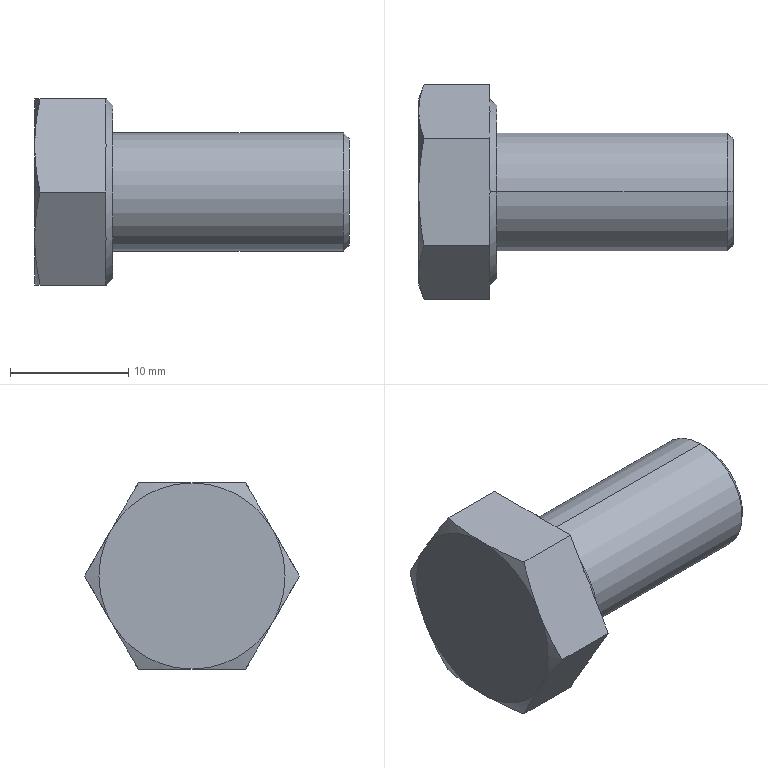Part | SolidWorks | features RevCut 3, Boss 1, Chamfer 1, Extrusion 1, Fillet 1, LPattern 1 | 1 solid | 27 faces | box 26.58 x 18.163 x 15.73 mm | volume 2955 mm3 | plane 15 | cone 10 | cylinder 2 | commonest cylinder face diameters 10 x2
STEP:
#1=CARTESIAN_POINT('',(26.58,0.,-4.5));
#2=VERTEX_POINT('',#1);
#3=CARTESIAN_POINT('',(26.58,0.,4.5));
#4=VERTEX_POINT('',#3);
#5=CARTESIAN_POINT('',(26.58,0.,0.));
#6=DIRECTION('',(1.,0.,0.));
#7=DIRECTION('',(0.,0.,-1.));
#8=AXIS2_PLACEMENT_3D('',#5,#6,#7);
#9=CIRCLE('',#8,4.5);
#10=EDGE_CURVE('',#2,#4,#9,.T.);
#11=ORIENTED_EDGE('',*,*,#10,.F.);
#12=CARTESIAN_POINT('',(26.08,0.,-5.));
#13=VERTEX_POINT('',#12);
#14=CARTESIAN_POINT('',(26.58,0.,-4.5));
#15=DIRECTION('',(-0.7071,0.,-0.7071));
#16=VECTOR('',#15,1000.);
#17=LINE('',#14,#16);
#18=EDGE_CURVE('',#2,#13,#17,.T.);
#19=ORIENTED_EDGE('',*,*,#18,.T.);
#20=CARTESIAN_POINT('',(26.08,0.,5.));
#21=VERTEX_POINT('',#20);
#22=CARTESIAN_POINT('',(26.08,0.,0.));
#23=DIRECTION('',(-1.,0.,0.));
#24=DIRECTION('',(0.,0.,-1.));
#25=AXIS2_PLACEMENT_3D('',#22,#23,#24);
#26=CIRCLE('',#25,5.);
#27=EDGE_CURVE('',#21,#13,#26,.T.);
#28=ORIENTED_EDGE('',*,*,#27,.F.);
#29=CARTESIAN_POINT('',(26.58,0.,4.5));
#30=DIRECTION('',(-0.7071,0.,0.7071));
#31=VECTOR('',#30,1000.);
#32=LINE('',#29,#31);
#33=EDGE_CURVE('',#4,#21,#32,.T.);
#34=ORIENTED_EDGE('',*,*,#33,.F.);
#35=EDGE_LOOP('',(#11,#19,#28,#34));
#36=FACE_OUTER_BOUND('',#35,.T.);
#37=CARTESIAN_POINT('',(26.58,0.,0.));
#38=DIRECTION('',(-1.,0.,0.));
#39=DIRECTION('',(0.,0.,1.));
#40=AXIS2_PLACEMENT_3D('',#37,#38,#39);
#41=CONICAL_SURFACE('',#40,4.5,0.7854);
#42=ADVANCED_FACE('',(#36),#41,.T.);
#43=ORIENTED_EDGE('',*,*,#27,.T.);
#44=CARTESIAN_POINT('',(6.58,0.,-5.));
#45=VERTEX_POINT('',#44);
#46=CARTESIAN_POINT('',(26.58,0.,-5.));
#47=DIRECTION('',(-1.,0.,0.));
#48=VECTOR('',#47,1000.);
#49=LINE('',#46,#48);
#50=EDGE_CURVE('',#13,#45,#49,.T.);
#51=ORIENTED_EDGE('',*,*,#50,.T.);
#52=CARTESIAN_POINT('',(6.58,0.,5.));
#53=VERTEX_POINT('',#52);
#54=CARTESIAN_POINT('',(6.58,0.,0.));
#55=DIRECTION('',(1.,0.,0.));
#56=DIRECTION('',(0.,0.,-1.));
#57=AXIS2_PLACEMENT_3D('',#54,#55,#56);
#58=CIRCLE('',#57,5.);
#59=EDGE_CURVE('',#45,#53,#58,.T.);
#60=ORIENTED_EDGE('',*,*,#59,.T.);
#61=CARTESIAN_POINT('',(26.58,0.,5.));
#62=DIRECTION('',(-1.,0.,0.));
#63=VECTOR('',#62,1000.);
#64=LINE('',#61,#63);
#65=EDGE_CURVE('',#21,#53,#64,.T.);
#66=ORIENTED_EDGE('',*,*,#65,.F.);
#67=EDGE_LOOP('',(#43,#51,#60,#66));
#68=FACE_OUTER_BOUND('',#67,.T.);
#69=CARTESIAN_POINT('',(26.58,0.,0.));
#70=DIRECTION('',(-1.,0.,0.));
#71=DIRECTION('',(0.,0.,1.));
#72=AXIS2_PLACEMENT_3D('',#69,#70,#71);
#73=CYLINDRICAL_SURFACE('',#72,5.);
#74=ADVANCED_FACE('',(#68),#73,.T.);
#75=CARTESIAN_POINT('',(6.58,0.,7.315));
#76=VERTEX_POINT('',#75);
#77=CARTESIAN_POINT('',(6.58,0.,-7.315));
#78=VERTEX_POINT('',#77);
#79=CARTESIAN_POINT('',(6.58,0.,0.));
#80=DIRECTION('',(-1.,0.,0.));
#81=DIRECTION('',(0.,0.,1.));
#82=AXIS2_PLACEMENT_3D('',#79,#80,#81);
#83=CIRCLE('',#82,7.315);
#84=EDGE_CURVE('',#76,#78,#83,.T.);
#85=ORIENTED_EDGE('',*,*,#84,.T.);
#86=CARTESIAN_POINT('',(6.03,0.,-7.865));
#87=VERTEX_POINT('',#86);
#88=CARTESIAN_POINT('',(5.98,0.,-7.915));
#89=DIRECTION('',(-0.7071,0.,-0.7071));
#90=VECTOR('',#89,1000.);
#91=LINE('',#88,#90);
#92=EDGE_CURVE('',#78,#87,#91,.T.);
#93=ORIENTED_EDGE('',*,*,#92,.T.);
#94=CARTESIAN_POINT('',(5.98,0.8883,-7.865));
#95=VERTEX_POINT('',#94);
#96=CARTESIAN_POINT('',(6.03,0.,-7.865));
#97=CARTESIAN_POINT('',(6.03,0.2963,-7.865));
#98=CARTESIAN_POINT('',(6.013,0.5924,-7.865));
#99=CARTESIAN_POINT('',(5.98,0.8883,-7.865));
#100=B_SPLINE_CURVE_WITH_KNOTS('',3,(#96,#97,#98,#99),.UNSPECIFIED.,.F.,.F.,(4,4),(0.004405,0.00529),.UNSPECIFIED.);
#101=EDGE_CURVE('',#87,#95,#100,.T.);
#102=ORIENTED_EDGE('',*,*,#101,.T.);
#103=CARTESIAN_POINT('',(5.98,6.367,-4.702));
#104=VERTEX_POINT('',#103);
#105=CARTESIAN_POINT('',(5.98,0.,0.));
#106=DIRECTION('',(-1.,0.,0.));
#107=DIRECTION('',(0.,0.,1.));
#108=AXIS2_PLACEMENT_3D('',#105,#106,#107);
#109=CIRCLE('',#108,7.915);
#110=EDGE_CURVE('',#104,#95,#109,.T.);
#111=ORIENTED_EDGE('',*,*,#110,.F.);
#112=CARTESIAN_POINT('',(5.98,7.255,-3.163));
#113=VERTEX_POINT('',#112);
#114=CARTESIAN_POINT('',(5.98,6.367,-4.702));
#115=CARTESIAN_POINT('',(6.046,6.663,-4.189));
#116=CARTESIAN_POINT('',(6.046,6.959,-3.676));
#117=CARTESIAN_POINT('',(5.98,7.255,-3.163));
#118=B_SPLINE_CURVE_WITH_KNOTS('',3,(#114,#115,#116,#117),.UNSPECIFIED.,.F.,.F.,(4,4),(0.00000178,0.001778),.UNSPECIFIED.);
#119=EDGE_CURVE('',#104,#113,#118,.T.);
#120=ORIENTED_EDGE('',*,*,#119,.T.);
#121=CARTESIAN_POINT('',(5.98,7.255,3.163));
#122=VERTEX_POINT('',#121);
#123=CARTESIAN_POINT('',(5.98,0.,0.));
#124=DIRECTION('',(-1.,0.,0.));
#125=DIRECTION('',(0.,0.,1.));
#126=AXIS2_PLACEMENT_3D('',#123,#124,#125);
#127=CIRCLE('',#126,7.915);
#128=EDGE_CURVE('',#122,#113,#127,.T.);
#129=ORIENTED_EDGE('',*,*,#128,.F.);
#130=CARTESIAN_POINT('',(5.98,6.367,4.702));
#131=VERTEX_POINT('',#130);
#132=CARTESIAN_POINT('',(5.98,7.255,3.163));
#133=CARTESIAN_POINT('',(6.046,6.959,3.676));
#134=CARTESIAN_POINT('',(6.046,6.663,4.189));
#135=CARTESIAN_POINT('',(5.98,6.367,4.702));
#136=B_SPLINE_CURVE_WITH_KNOTS('',3,(#132,#133,#134,#135),.UNSPECIFIED.,.F.,.F.,(4,4),(0.00000178,0.001778),.UNSPECIFIED.);
#137=EDGE_CURVE('',#122,#131,#136,.T.);
#138=ORIENTED_EDGE('',*,*,#137,.T.);
#139=CARTESIAN_POINT('',(5.98,0.8883,7.865));
#140=VERTEX_POINT('',#139);
#141=CARTESIAN_POINT('',(5.98,0.,0.));
#142=DIRECTION('',(-1.,0.,0.));
#143=DIRECTION('',(0.,0.,1.));
#144=AXIS2_PLACEMENT_3D('',#141,#142,#143);
#145=CIRCLE('',#144,7.915);
#146=EDGE_CURVE('',#140,#131,#145,.T.);
#147=ORIENTED_EDGE('',*,*,#146,.F.);
#148=CARTESIAN_POINT('',(6.03,0.,7.865));
#149=VERTEX_POINT('',#148);
#150=CARTESIAN_POINT('',(5.98,0.8883,7.865));
#151=CARTESIAN_POINT('',(6.013,0.5924,7.865));
#152=CARTESIAN_POINT('',(6.03,0.2963,7.865));
#153=CARTESIAN_POINT('',(6.03,0.,7.865));
#154=B_SPLINE_CURVE_WITH_KNOTS('',3,(#150,#151,#152,#153),.UNSPECIFIED.,.F.,.F.,(4,4),(0.003909,0.004793),.UNSPECIFIED.);
#155=EDGE_CURVE('',#140,#149,#154,.T.);
#156=ORIENTED_EDGE('',*,*,#155,.T.);
#157=CARTESIAN_POINT('',(5.98,0.,7.915));
#158=DIRECTION('',(-0.7071,0.,0.7071));
#159=VECTOR('',#158,1000.);
#160=LINE('',#157,#159);
#161=EDGE_CURVE('',#76,#149,#160,.T.);
#162=ORIENTED_EDGE('',*,*,#161,.F.);
#163=EDGE_LOOP('',(#85,#93,#102,#111,#120,#129,#138,#147,#156,#162));
#164=FACE_OUTER_BOUND('',#163,.T.);
#165=CARTESIAN_POINT('',(5.98,0.,0.));
#166=DIRECTION('',(-1.,0.,0.));
#167=DIRECTION('',(0.,0.,1.));
#168=AXIS2_PLACEMENT_3D('',#165,#166,#167);
#169=CONICAL_SURFACE('',#168,7.915,0.7854);
#170=ADVANCED_FACE('',(#164),#169,.T.);
#171=ORIENTED_EDGE('',*,*,#84,.F.);
#172=CARTESIAN_POINT('',(6.58,0.,0.));
#173=DIRECTION('',(-1.,0.,0.));
#174=DIRECTION('',(0.,0.,1.));
#175=AXIS2_PLACEMENT_3D('',#172,#173,#174);
#176=CIRCLE('',#175,7.315);
#177=EDGE_CURVE('',#78,#76,#176,.T.);
#178=ORIENTED_EDGE('',*,*,#177,.F.);
#179=EDGE_LOOP('',(#171,#178));
#180=FACE_OUTER_BOUND('',#179,.T.);
#181=CARTESIAN_POINT('',(6.58,0.,0.));
#182=DIRECTION('',(1.,0.,0.));
#183=DIRECTION('',(0.,0.,-1.));
#184=AXIS2_PLACEMENT_3D('',#181,#182,#183);
#185=CIRCLE('',#184,5.);
#186=EDGE_CURVE('',#53,#45,#185,.T.);
#187=ORIENTED_EDGE('',*,*,#186,.F.);
#188=ORIENTED_EDGE('',*,*,#59,.F.);
#189=EDGE_LOOP('',(#187,#188));
#190=FACE_BOUND('',#189,.T.);
#191=CARTESIAN_POINT('',(6.58,-4.541,-7.865));
#192=DIRECTION('',(1.,0.,0.));
#193=DIRECTION('',(0.,0.,-1.));
#194=AXIS2_PLACEMENT_3D('',#191,#192,#193);
#195=PLANE('',#194);
#196=ADVANCED_FACE('',(#180,#190),#195,.T.);
#197=CARTESIAN_POINT('',(0.4428,-4.541,-7.865));
#198=VERTEX_POINT('',#197);
#199=CARTESIAN_POINT('',(0.,-6.811,-3.932));
#200=VERTEX_POINT('',#199);
#201=CARTESIAN_POINT('',(0.4428,-4.541,-7.865));
#202=CARTESIAN_POINT('',(0.3051,-4.919,-7.21));
#203=CARTESIAN_POINT('',(0.1933,-5.298,-6.554));
#204=CARTESIAN_POINT('',(0.04049,-6.054,-5.243));
#205=CARTESIAN_POINT('',(0.,-6.433,-4.588));
#206=CARTESIAN_POINT('',(0.,-6.811,-3.932));
#207=B_SPLINE_CURVE_WITH_KNOTS('',3,(#201,#202,#203,#204,#205,#206),.UNSPECIFIED.,.F.,.F.,(4,2,4),(0.000000231,0.002271,0.004541),.UNSPECIFIED.);
#208=EDGE_CURVE('',#198,#200,#207,.T.);
#209=ORIENTED_EDGE('',*,*,#208,.F.);
#210=CARTESIAN_POINT('',(5.98,-4.541,-7.865));
#211=VERTEX_POINT('',#210);
#212=CARTESIAN_POINT('',(6.58,-4.541,-7.865));
#213=DIRECTION('',(-1.,0.,0.));
#214=VECTOR('',#213,1000.);
#215=LINE('',#212,#214);
#216=EDGE_CURVE('',#211,#198,#215,.T.);
#217=ORIENTED_EDGE('',*,*,#216,.F.);
#218=CARTESIAN_POINT('',(5.98,-6.367,-4.702));
#219=VERTEX_POINT('',#218);
#220=CARTESIAN_POINT('',(5.98,-9.082,0.));
#221=DIRECTION('',(0.,0.5,-0.866));
#222=VECTOR('',#221,1000.);
#223=LINE('',#220,#222);
#224=EDGE_CURVE('',#219,#211,#223,.T.);
#225=ORIENTED_EDGE('',*,*,#224,.F.);
#226=CARTESIAN_POINT('',(5.98,-7.255,-3.163));
#227=VERTEX_POINT('',#226);
#228=CARTESIAN_POINT('',(5.98,-7.255,-3.163));
#229=CARTESIAN_POINT('',(6.046,-6.959,-3.676));
#230=CARTESIAN_POINT('',(6.046,-6.663,-4.189));
#231=CARTESIAN_POINT('',(5.98,-6.367,-4.702));
#232=B_SPLINE_CURVE_WITH_KNOTS('',3,(#228,#229,#230,#231),.UNSPECIFIED.,.F.,.F.,(4,4),(0.00000178,0.001778),.UNSPECIFIED.);
#233=EDGE_CURVE('',#227,#219,#232,.T.);
#234=ORIENTED_EDGE('',*,*,#233,.F.);
#235=CARTESIAN_POINT('',(5.98,-9.082,0.));
#236=VERTEX_POINT('',#235);
#237=CARTESIAN_POINT('',(5.98,-9.082,0.));
#238=DIRECTION('',(0.,0.5,-0.866));
#239=VECTOR('',#238,1000.);
#240=LINE('',#237,#239);
#241=EDGE_CURVE('',#236,#227,#240,.T.);
#242=ORIENTED_EDGE('',*,*,#241,.F.);
#243=CARTESIAN_POINT('',(0.4428,-9.082,0.));
#244=VERTEX_POINT('',#243);
#245=CARTESIAN_POINT('',(6.58,-9.082,0.));
#246=DIRECTION('',(-1.,0.,0.));
#247=VECTOR('',#246,1000.);
#248=LINE('',#245,#247);
#249=EDGE_CURVE('',#236,#244,#248,.T.);
#250=ORIENTED_EDGE('',*,*,#249,.T.);
#251=CARTESIAN_POINT('',(0.,-6.811,-3.932));
#252=CARTESIAN_POINT('',(0.,-7.19,-3.277));
#253=CARTESIAN_POINT('',(0.04049,-7.568,-2.622));
#254=CARTESIAN_POINT('',(0.1933,-8.325,-1.311));
#255=CARTESIAN_POINT('',(0.3051,-8.703,-0.6554));
#256=CARTESIAN_POINT('',(0.4428,-9.082,0.));
#257=B_SPLINE_CURVE_WITH_KNOTS('',3,(#251,#252,#253,#254,#255,#256),.UNSPECIFIED.,.F.,.F.,(4,2,4),(0.004541,0.006812,0.009082),.UNSPECIFIED.);
#258=EDGE_CURVE('',#200,#244,#257,.T.);
#259=ORIENTED_EDGE('',*,*,#258,.F.);
#260=EDGE_LOOP('',(#209,#217,#225,#234,#242,#250,#259));
#261=FACE_OUTER_BOUND('',#260,.T.);
#262=CARTESIAN_POINT('',(6.58,-9.082,0.));
#263=DIRECTION('',(0.,0.866,0.5));
#264=DIRECTION('',(0.,-0.5,0.866));
#265=AXIS2_PLACEMENT_3D('',#262,#263,#264);
#266=PLANE('',#265);
#267=ADVANCED_FACE('',(#261),#266,.F.);
#268=CARTESIAN_POINT('',(0.4428,4.541,-7.865));
#269=VERTEX_POINT('',#268);
#270=CARTESIAN_POINT('',(0.,0.,-7.865));
#271=VERTEX_POINT('',#270);
#272=CARTESIAN_POINT('',(0.4428,4.541,-7.865));
#273=CARTESIAN_POINT('',(0.3055,3.786,-7.865));
#274=CARTESIAN_POINT('',(0.1936,3.029,-7.865));
#275=CARTESIAN_POINT('',(0.04065,1.516,-7.865));
#276=CARTESIAN_POINT('',(0.,0.7584,-7.865));
#277=CARTESIAN_POINT('',(0.,0.,-7.865));
#278=B_SPLINE_CURVE_WITH_KNOTS('',3,(#272,#273,#274,#275,#276,#277),.UNSPECIFIED.,.F.,.F.,(4,2,4),(0.01637,0.01866,0.02095),.UNSPECIFIED.);
#279=EDGE_CURVE('',#269,#271,#278,.T.);
#280=ORIENTED_EDGE('',*,*,#279,.F.);
#281=CARTESIAN_POINT('',(5.98,4.541,-7.865));
#282=VERTEX_POINT('',#281);
#283=CARTESIAN_POINT('',(6.58,4.541,-7.865));
#284=DIRECTION('',(-1.,0.,0.));
#285=VECTOR('',#284,1000.);
#286=LINE('',#283,#285);
#287=EDGE_CURVE('',#282,#269,#286,.T.);
#288=ORIENTED_EDGE('',*,*,#287,.F.);
#289=CARTESIAN_POINT('',(5.98,-4.541,-7.865));
#290=DIRECTION('',(0.,1.,0.));
#291=VECTOR('',#290,1000.);
#292=LINE('',#289,#291);
#293=EDGE_CURVE('',#95,#282,#292,.T.);
#294=ORIENTED_EDGE('',*,*,#293,.F.);
#295=ORIENTED_EDGE('',*,*,#101,.F.);
#296=CARTESIAN_POINT('',(5.98,-0.8883,-7.865));
#297=VERTEX_POINT('',#296);
#298=CARTESIAN_POINT('',(5.98,-0.8883,-7.865));
#299=CARTESIAN_POINT('',(6.013,-0.592,-7.865));
#300=CARTESIAN_POINT('',(6.03,-0.2959,-7.865));
#301=CARTESIAN_POINT('',(6.03,0.,-7.865));
#302=B_SPLINE_CURVE_WITH_KNOTS('',3,(#298,#299,#300,#301),.UNSPECIFIED.,.F.,.F.,(4,4),(0.00352,0.004405),.UNSPECIFIED.);
#303=EDGE_CURVE('',#297,#87,#302,.T.);
#304=ORIENTED_EDGE('',*,*,#303,.F.);
#305=CARTESIAN_POINT('',(5.98,-4.541,-7.865));
#306=DIRECTION('',(0.,1.,0.));
#307=VECTOR('',#306,1000.);
#308=LINE('',#305,#307);
#309=EDGE_CURVE('',#211,#297,#308,.T.);
#310=ORIENTED_EDGE('',*,*,#309,.F.);
#311=ORIENTED_EDGE('',*,*,#216,.T.);
#312=CARTESIAN_POINT('',(0.,0.,-7.865));
#313=CARTESIAN_POINT('',(0.,-0.7562,-7.865));
#314=CARTESIAN_POINT('',(0.04043,-1.513,-7.865));
#315=CARTESIAN_POINT('',(0.1935,-3.029,-7.865));
#316=CARTESIAN_POINT('',(0.306,-3.789,-7.865));
#317=CARTESIAN_POINT('',(0.4428,-4.541,-7.865));
#318=B_SPLINE_CURVE_WITH_KNOTS('',3,(#312,#313,#314,#315,#316,#317),.UNSPECIFIED.,.F.,.F.,(4,2,4),(0.02095,0.02323,0.02552),.UNSPECIFIED.);
#319=EDGE_CURVE('',#271,#198,#318,.T.);
#320=ORIENTED_EDGE('',*,*,#319,.F.);
#321=EDGE_LOOP('',(#280,#288,#294,#295,#304,#310,#311,#320));
#322=FACE_OUTER_BOUND('',#321,.T.);
#323=CARTESIAN_POINT('',(6.58,-4.541,-7.865));
#324=DIRECTION('',(0.,0.,1.));
#325=DIRECTION('',(1.,0.,0.));
#326=AXIS2_PLACEMENT_3D('',#323,#324,#325);
#327=PLANE('',#326);
#328=ADVANCED_FACE('',(#322),#327,.F.);
#329=CARTESIAN_POINT('',(0.4428,9.082,0.));
#330=VERTEX_POINT('',#329);
#331=CARTESIAN_POINT('',(0.,6.811,-3.933));
#332=VERTEX_POINT('',#331);
#333=CARTESIAN_POINT('',(0.4428,9.082,0.));
#334=CARTESIAN_POINT('',(0.3051,8.703,-0.6554));
#335=CARTESIAN_POINT('',(0.1933,8.325,-1.311));
#336=CARTESIAN_POINT('',(0.04049,7.568,-2.622));
#337=CARTESIAN_POINT('',(0.,7.19,-3.277));
#338=CARTESIAN_POINT('',(0.,6.811,-3.933));
#339=B_SPLINE_CURVE_WITH_KNOTS('',3,(#333,#334,#335,#336,#337,#338),.UNSPECIFIED.,.F.,.F.,(4,2,4),(0.000000231,0.002271,0.004541),.UNSPECIFIED.);
#340=EDGE_CURVE('',#330,#332,#339,.T.);
#341=ORIENTED_EDGE('',*,*,#340,.F.);
#342=CARTESIAN_POINT('',(5.98,9.082,0.));
#343=VERTEX_POINT('',#342);
#344=CARTESIAN_POINT('',(6.58,9.082,0.));
#345=DIRECTION('',(-1.,0.,0.));
#346=VECTOR('',#345,1000.);
#347=LINE('',#344,#346);
#348=EDGE_CURVE('',#343,#330,#347,.T.);
#349=ORIENTED_EDGE('',*,*,#348,.F.);
#350=CARTESIAN_POINT('',(5.98,4.541,-7.865));
#351=DIRECTION('',(0.,0.5,0.866));
#352=VECTOR('',#351,1000.);
#353=LINE('',#350,#352);
#354=EDGE_CURVE('',#113,#343,#353,.T.);
#355=ORIENTED_EDGE('',*,*,#354,.F.);
#356=ORIENTED_EDGE('',*,*,#119,.F.);
#357=CARTESIAN_POINT('',(5.98,4.541,-7.865));
#358=DIRECTION('',(0.,0.5,0.866));
#359=VECTOR('',#358,1000.);
#360=LINE('',#357,#359);
#361=EDGE_CURVE('',#282,#104,#360,.T.);
#362=ORIENTED_EDGE('',*,*,#361,.F.);
#363=ORIENTED_EDGE('',*,*,#287,.T.);
#364=CARTESIAN_POINT('',(0.,6.811,-3.933));
#365=CARTESIAN_POINT('',(0.,6.433,-4.588));
#366=CARTESIAN_POINT('',(0.04049,6.054,-5.243));
#367=CARTESIAN_POINT('',(0.1933,5.298,-6.554));
#368=CARTESIAN_POINT('',(0.3051,4.919,-7.21));
#369=CARTESIAN_POINT('',(0.4428,4.541,-7.865));
#370=B_SPLINE_CURVE_WITH_KNOTS('',3,(#364,#365,#366,#367,#368,#369),.UNSPECIFIED.,.F.,.F.,(4,2,4),(0.004541,0.006812,0.009082),.UNSPECIFIED.);
#371=EDGE_CURVE('',#332,#269,#370,.T.);
#372=ORIENTED_EDGE('',*,*,#371,.F.);
#373=EDGE_LOOP('',(#341,#349,#355,#356,#362,#363,#372));
#374=FACE_OUTER_BOUND('',#373,.T.);
#375=CARTESIAN_POINT('',(6.58,4.541,-7.865));
#376=DIRECTION('',(0.,-0.866,0.5));
#377=DIRECTION('',(0.,-0.5,-0.866));
#378=AXIS2_PLACEMENT_3D('',#375,#376,#377);
#379=PLANE('',#378);
#380=ADVANCED_FACE('',(#374),#379,.F.);
#381=CARTESIAN_POINT('',(0.4428,4.541,7.865));
#382=VERTEX_POINT('',#381);
#383=CARTESIAN_POINT('',(0.,6.811,3.932));
#384=VERTEX_POINT('',#383);
#385=CARTESIAN_POINT('',(0.4428,4.541,7.865));
#386=CARTESIAN_POINT('',(0.3051,4.919,7.21));
#387=CARTESIAN_POINT('',(0.1933,5.298,6.554));
#388=CARTESIAN_POINT('',(0.04049,6.054,5.243));
#389=CARTESIAN_POINT('',(0.,6.433,4.588));
#390=CARTESIAN_POINT('',(0.,6.811,3.932));
#391=B_SPLINE_CURVE_WITH_KNOTS('',3,(#385,#386,#387,#388,#389,#390),.UNSPECIFIED.,.F.,.F.,(4,2,4),(0.000000231,0.002271,0.004541),.UNSPECIFIED.);
#392=EDGE_CURVE('',#382,#384,#391,.T.);
#393=ORIENTED_EDGE('',*,*,#392,.F.);
#394=CARTESIAN_POINT('',(5.98,4.541,7.865));
#395=VERTEX_POINT('',#394);
#396=CARTESIAN_POINT('',(6.58,4.541,7.865));
#397=DIRECTION('',(-1.,0.,0.));
#398=VECTOR('',#397,1000.);
#399=LINE('',#396,#398);
#400=EDGE_CURVE('',#395,#382,#399,.T.);
#401=ORIENTED_EDGE('',*,*,#400,.F.);
#402=CARTESIAN_POINT('',(5.98,9.082,0.));
#403=DIRECTION('',(0.,-0.5,0.866));
#404=VECTOR('',#403,1000.);
#405=LINE('',#402,#404);
#406=EDGE_CURVE('',#131,#395,#405,.T.);
#407=ORIENTED_EDGE('',*,*,#406,.F.);
#408=ORIENTED_EDGE('',*,*,#137,.F.);
#409=CARTESIAN_POINT('',(5.98,9.082,0.));
#410=DIRECTION('',(0.,-0.5,0.866));
#411=VECTOR('',#410,1000.);
#412=LINE('',#409,#411);
#413=EDGE_CURVE('',#343,#122,#412,.T.);
#414=ORIENTED_EDGE('',*,*,#413,.F.);
#415=ORIENTED_EDGE('',*,*,#348,.T.);
#416=CARTESIAN_POINT('',(0.,6.811,3.932));
#417=CARTESIAN_POINT('',(0.,7.19,3.277));
#418=CARTESIAN_POINT('',(0.04049,7.568,2.622));
#419=CARTESIAN_POINT('',(0.1933,8.325,1.311));
#420=CARTESIAN_POINT('',(0.3051,8.703,0.6554));
#421=CARTESIAN_POINT('',(0.4428,9.082,0.));
#422=B_SPLINE_CURVE_WITH_KNOTS('',3,(#416,#417,#418,#419,#420,#421),.UNSPECIFIED.,.F.,.F.,(4,2,4),(0.004541,0.006812,0.009082),.UNSPECIFIED.);
#423=EDGE_CURVE('',#384,#330,#422,.T.);
#424=ORIENTED_EDGE('',*,*,#423,.F.);
#425=EDGE_LOOP('',(#393,#401,#407,#408,#414,#415,#424));
#426=FACE_OUTER_BOUND('',#425,.T.);
#427=CARTESIAN_POINT('',(6.58,9.082,0.));
#428=DIRECTION('',(0.,-0.866,-0.5));
#429=DIRECTION('',(0.,0.5,-0.866));
#430=AXIS2_PLACEMENT_3D('',#427,#428,#429);
#431=PLANE('',#430);
#432=ADVANCED_FACE('',(#426),#431,.F.);
#433=CARTESIAN_POINT('',(0.4428,-4.541,7.865));
#434=VERTEX_POINT('',#433);
#435=CARTESIAN_POINT('',(0.,0.,7.865));
#436=VERTEX_POINT('',#435);
#437=CARTESIAN_POINT('',(0.4428,-4.541,7.865));
#438=CARTESIAN_POINT('',(0.306,-3.789,7.865));
#439=CARTESIAN_POINT('',(0.1935,-3.029,7.865));
#440=CARTESIAN_POINT('',(0.04043,-1.513,7.865));
#441=CARTESIAN_POINT('',(0.,-0.7562,7.865));
#442=CARTESIAN_POINT('',(0.,0.,7.865));
#443=B_SPLINE_CURVE_WITH_KNOTS('',3,(#437,#438,#439,#440,#441,#442),.UNSPECIFIED.,.F.,.F.,(4,2,4),(0.007725,0.01001,0.0123),.UNSPECIFIED.);
#444=EDGE_CURVE('',#434,#436,#443,.T.);
#445=ORIENTED_EDGE('',*,*,#444,.F.);
#446=CARTESIAN_POINT('',(5.98,-4.541,7.865));
#447=VERTEX_POINT('',#446);
#448=CARTESIAN_POINT('',(6.58,-4.541,7.865));
#449=DIRECTION('',(-1.,0.,0.));
#450=VECTOR('',#449,1000.);
#451=LINE('',#448,#450);
#452=EDGE_CURVE('',#447,#434,#451,.T.);
#453=ORIENTED_EDGE('',*,*,#452,.F.);
#454=CARTESIAN_POINT('',(5.98,-0.8883,7.865));
#455=VERTEX_POINT('',#454);
#456=CARTESIAN_POINT('',(5.98,4.541,7.865));
#457=DIRECTION('',(0.,-1.,0.));
#458=VECTOR('',#457,1000.);
#459=LINE('',#456,#458);
#460=EDGE_CURVE('',#455,#447,#459,.T.);
#461=ORIENTED_EDGE('',*,*,#460,.F.);
#462=CARTESIAN_POINT('',(6.03,0.,7.865));
#463=CARTESIAN_POINT('',(6.03,-0.2959,7.865));
#464=CARTESIAN_POINT('',(6.013,-0.592,7.865));
#465=CARTESIAN_POINT('',(5.98,-0.8883,7.865));
#466=B_SPLINE_CURVE_WITH_KNOTS('',3,(#462,#463,#464,#465),.UNSPECIFIED.,.F.,.F.,(4,4),(0.004793,0.005677),.UNSPECIFIED.);
#467=EDGE_CURVE('',#149,#455,#466,.T.);
#468=ORIENTED_EDGE('',*,*,#467,.F.);
#469=ORIENTED_EDGE('',*,*,#155,.F.);
#470=CARTESIAN_POINT('',(5.98,4.541,7.865));
#471=DIRECTION('',(0.,-1.,0.));
#472=VECTOR('',#471,1000.);
#473=LINE('',#470,#472);
#474=EDGE_CURVE('',#395,#140,#473,.T.);
#475=ORIENTED_EDGE('',*,*,#474,.F.);
#476=ORIENTED_EDGE('',*,*,#400,.T.);
#477=CARTESIAN_POINT('',(0.,0.,7.865));
#478=CARTESIAN_POINT('',(0.,0.7584,7.865));
#479=CARTESIAN_POINT('',(0.04065,1.516,7.865));
#480=CARTESIAN_POINT('',(0.1936,3.029,7.865));
#481=CARTESIAN_POINT('',(0.3055,3.786,7.865));
#482=CARTESIAN_POINT('',(0.4428,4.541,7.865));
#483=B_SPLINE_CURVE_WITH_KNOTS('',3,(#477,#478,#479,#480,#481,#482),.UNSPECIFIED.,.F.,.F.,(4,2,4),(0.0123,0.0146,0.01689),.UNSPECIFIED.);
#484=EDGE_CURVE('',#436,#382,#483,.T.);
#485=ORIENTED_EDGE('',*,*,#484,.F.);
#486=EDGE_LOOP('',(#445,#453,#461,#468,#469,#475,#476,#485));
#487=FACE_OUTER_BOUND('',#486,.T.);
#488=CARTESIAN_POINT('',(6.58,4.541,7.865));
#489=DIRECTION('',(0.,0.,-1.));
#490=DIRECTION('',(-1.,0.,0.));
#491=AXIS2_PLACEMENT_3D('',#488,#489,#490);
#492=PLANE('',#491);
#493=ADVANCED_FACE('',(#487),#492,.F.);
#494=CARTESIAN_POINT('',(0.,-6.811,3.932));
#495=VERTEX_POINT('',#494);
#496=CARTESIAN_POINT('',(0.4428,-9.082,0.));
#497=CARTESIAN_POINT('',(0.3051,-8.703,0.6554));
#498=CARTESIAN_POINT('',(0.1933,-8.325,1.311));
#499=CARTESIAN_POINT('',(0.04049,-7.568,2.622));
#500=CARTESIAN_POINT('',(0.,-7.19,3.277));
#501=CARTESIAN_POINT('',(0.,-6.811,3.932));
#502=B_SPLINE_CURVE_WITH_KNOTS('',3,(#496,#497,#498,#499,#500,#501),.UNSPECIFIED.,.F.,.F.,(4,2,4),(0.000000231,0.002271,0.004541),.UNSPECIFIED.);
#503=EDGE_CURVE('',#244,#495,#502,.T.);
#504=ORIENTED_EDGE('',*,*,#503,.F.);
#505=ORIENTED_EDGE('',*,*,#249,.F.);
#506=CARTESIAN_POINT('',(5.98,-7.255,3.163));
#507=VERTEX_POINT('',#506);
#508=CARTESIAN_POINT('',(5.98,-4.541,7.865));
#509=DIRECTION('',(0.,-0.5,-0.866));
#510=VECTOR('',#509,1000.);
#511=LINE('',#508,#510);
#512=EDGE_CURVE('',#507,#236,#511,.T.);
#513=ORIENTED_EDGE('',*,*,#512,.F.);
#514=CARTESIAN_POINT('',(5.98,-6.367,4.702));
#515=VERTEX_POINT('',#514);
#516=CARTESIAN_POINT('',(5.98,-6.367,4.702));
#517=CARTESIAN_POINT('',(6.046,-6.663,4.189));
#518=CARTESIAN_POINT('',(6.046,-6.959,3.676));
#519=CARTESIAN_POINT('',(5.98,-7.255,3.163));
#520=B_SPLINE_CURVE_WITH_KNOTS('',3,(#516,#517,#518,#519),.UNSPECIFIED.,.F.,.F.,(4,4),(0.00000178,0.001778),.UNSPECIFIED.);
#521=EDGE_CURVE('',#515,#507,#520,.T.);
#522=ORIENTED_EDGE('',*,*,#521,.F.);
#523=CARTESIAN_POINT('',(5.98,-4.541,7.865));
#524=DIRECTION('',(0.,-0.5,-0.866));
#525=VECTOR('',#524,1000.);
#526=LINE('',#523,#525);
#527=EDGE_CURVE('',#447,#515,#526,.T.);
#528=ORIENTED_EDGE('',*,*,#527,.F.);
#529=ORIENTED_EDGE('',*,*,#452,.T.);
#530=CARTESIAN_POINT('',(0.,-6.811,3.932));
#531=CARTESIAN_POINT('',(0.,-6.433,4.588));
#532=CARTESIAN_POINT('',(0.04049,-6.054,5.243));
#533=CARTESIAN_POINT('',(0.1933,-5.298,6.554));
#534=CARTESIAN_POINT('',(0.3051,-4.919,7.21));
#535=CARTESIAN_POINT('',(0.4428,-4.541,7.865));
#536=B_SPLINE_CURVE_WITH_KNOTS('',3,(#530,#531,#532,#533,#534,#535),.UNSPECIFIED.,.F.,.F.,(4,2,4),(0.004541,0.006812,0.009082),.UNSPECIFIED.);
#537=EDGE_CURVE('',#495,#434,#536,.T.);
#538=ORIENTED_EDGE('',*,*,#537,.F.);
#539=EDGE_LOOP('',(#504,#505,#513,#522,#528,#529,#538));
#540=FACE_OUTER_BOUND('',#539,.T.);
#541=CARTESIAN_POINT('',(6.58,-4.541,7.865));
#542=DIRECTION('',(0.,0.866,-0.5));
#543=DIRECTION('',(0.,0.5,0.866));
#544=AXIS2_PLACEMENT_3D('',#541,#542,#543);
#545=PLANE('',#544);
#546=ADVANCED_FACE('',(#540),#545,.F.);
#547=ORIENTED_EDGE('',*,*,#224,.T.);
#548=ORIENTED_EDGE('',*,*,#309,.T.);
#549=CARTESIAN_POINT('',(5.98,0.,0.));
#550=DIRECTION('',(-1.,0.,0.));
#551=DIRECTION('',(0.,0.,1.));
#552=AXIS2_PLACEMENT_3D('',#549,#550,#551);
#553=CIRCLE('',#552,7.915);
#554=EDGE_CURVE('',#297,#219,#553,.T.);
#555=ORIENTED_EDGE('',*,*,#554,.T.);
#556=EDGE_LOOP('',(#547,#548,#555));
#557=FACE_OUTER_BOUND('',#556,.T.);
#558=CARTESIAN_POINT('',(5.98,7.915,0.));
#559=DIRECTION('',(1.,0.,0.));
#560=DIRECTION('',(0.,0.,-1.));
#561=AXIS2_PLACEMENT_3D('',#558,#559,#560);
#562=PLANE('',#561);
#563=ADVANCED_FACE('',(#557),#562,.T.);
#564=ORIENTED_EDGE('',*,*,#293,.T.);
#565=ORIENTED_EDGE('',*,*,#361,.T.);
#566=ORIENTED_EDGE('',*,*,#110,.T.);
#567=EDGE_LOOP('',(#564,#565,#566));
#568=FACE_OUTER_BOUND('',#567,.T.);
#569=CARTESIAN_POINT('',(5.98,7.915,0.));
#570=DIRECTION('',(1.,0.,0.));
#571=DIRECTION('',(0.,0.,-1.));
#572=AXIS2_PLACEMENT_3D('',#569,#570,#571);
#573=PLANE('',#572);
#574=ADVANCED_FACE('',(#568),#573,.T.);
#575=ORIENTED_EDGE('',*,*,#354,.T.);
#576=ORIENTED_EDGE('',*,*,#413,.T.);
#577=ORIENTED_EDGE('',*,*,#128,.T.);
#578=EDGE_LOOP('',(#575,#576,#577));
#579=FACE_OUTER_BOUND('',#578,.T.);
#580=CARTESIAN_POINT('',(5.98,7.915,0.));
#581=DIRECTION('',(1.,0.,0.));
#582=DIRECTION('',(0.,0.,-1.));
#583=AXIS2_PLACEMENT_3D('',#580,#581,#582);
#584=PLANE('',#583);
#585=ADVANCED_FACE('',(#579),#584,.T.);
#586=ORIENTED_EDGE('',*,*,#406,.T.);
#587=ORIENTED_EDGE('',*,*,#474,.T.);
#588=ORIENTED_EDGE('',*,*,#146,.T.);
#589=EDGE_LOOP('',(#586,#587,#588));
#590=FACE_OUTER_BOUND('',#589,.T.);
#591=CARTESIAN_POINT('',(5.98,7.915,0.));
#592=DIRECTION('',(1.,0.,0.));
#593=DIRECTION('',(0.,0.,-1.));
#594=AXIS2_PLACEMENT_3D('',#591,#592,#593);
#595=PLANE('',#594);
#596=ADVANCED_FACE('',(#590),#595,.T.);
#597=ORIENTED_EDGE('',*,*,#460,.T.);
#598=ORIENTED_EDGE('',*,*,#527,.T.);
#599=CARTESIAN_POINT('',(5.98,0.,0.));
#600=DIRECTION('',(-1.,0.,0.));
#601=DIRECTION('',(0.,0.,1.));
#602=AXIS2_PLACEMENT_3D('',#599,#600,#601);
#603=CIRCLE('',#602,7.915);
#604=EDGE_CURVE('',#515,#455,#603,.T.);
#605=ORIENTED_EDGE('',*,*,#604,.T.);
#606=EDGE_LOOP('',(#597,#598,#605));
#607=FACE_OUTER_BOUND('',#606,.T.);
#608=CARTESIAN_POINT('',(5.98,7.915,0.));
#609=DIRECTION('',(1.,0.,0.));
#610=DIRECTION('',(0.,0.,-1.));
#611=AXIS2_PLACEMENT_3D('',#608,#609,#610);
#612=PLANE('',#611);
#613=ADVANCED_FACE('',(#607),#612,.T.);
#614=ORIENTED_EDGE('',*,*,#241,.T.);
#615=CARTESIAN_POINT('',(5.98,0.,0.));
#616=DIRECTION('',(-1.,0.,0.));
#617=DIRECTION('',(0.,0.,1.));
#618=AXIS2_PLACEMENT_3D('',#615,#616,#617);
#619=CIRCLE('',#618,7.915);
#620=EDGE_CURVE('',#227,#507,#619,.T.);
#621=ORIENTED_EDGE('',*,*,#620,.T.);
#622=ORIENTED_EDGE('',*,*,#512,.T.);
#623=EDGE_LOOP('',(#614,#621,#622));
#624=FACE_OUTER_BOUND('',#623,.T.);
#625=CARTESIAN_POINT('',(5.98,7.915,0.));
#626=DIRECTION('',(1.,0.,0.));
#627=DIRECTION('',(0.,0.,-1.));
#628=AXIS2_PLACEMENT_3D('',#625,#626,#627);
#629=PLANE('',#628);
#630=ADVANCED_FACE('',(#624),#629,.T.);
#631=ORIENTED_EDGE('',*,*,#92,.F.);
#632=ORIENTED_EDGE('',*,*,#177,.T.);
#633=ORIENTED_EDGE('',*,*,#161,.T.);
#634=ORIENTED_EDGE('',*,*,#467,.T.);
#635=ORIENTED_EDGE('',*,*,#604,.F.);
#636=ORIENTED_EDGE('',*,*,#521,.T.);
#637=ORIENTED_EDGE('',*,*,#620,.F.);
#638=ORIENTED_EDGE('',*,*,#233,.T.);
#639=ORIENTED_EDGE('',*,*,#554,.F.);
#640=ORIENTED_EDGE('',*,*,#303,.T.);
#641=EDGE_LOOP('',(#631,#632,#633,#634,#635,#636,#637,#638,#639,#640));
#642=FACE_OUTER_BOUND('',#641,.T.);
#643=CARTESIAN_POINT('',(5.98,0.,0.));
#644=DIRECTION('',(-1.,0.,0.));
#645=DIRECTION('',(0.,0.,1.));
#646=AXIS2_PLACEMENT_3D('',#643,#644,#645);
#647=CONICAL_SURFACE('',#646,7.915,0.7854);
#648=ADVANCED_FACE('',(#642),#647,.T.);
#649=ORIENTED_EDGE('',*,*,#319,.T.);
#650=ORIENTED_EDGE('',*,*,#208,.T.);
#651=CARTESIAN_POINT('',(0.,0.,0.));
#652=DIRECTION('',(1.,0.,0.));
#653=DIRECTION('',(0.,0.,-1.));
#654=AXIS2_PLACEMENT_3D('',#651,#652,#653);
#655=CIRCLE('',#654,7.865);
#656=EDGE_CURVE('',#200,#271,#655,.T.);
#657=ORIENTED_EDGE('',*,*,#656,.T.);
#658=EDGE_LOOP('',(#649,#650,#657));
#659=FACE_OUTER_BOUND('',#658,.T.);
#660=CARTESIAN_POINT('',(0.,0.,0.));
#661=DIRECTION('',(1.,0.,0.));
#662=DIRECTION('',(0.,0.,-1.));
#663=AXIS2_PLACEMENT_3D('',#660,#661,#662);
#664=CONICAL_SURFACE('',#663,7.865,1.222);
#665=ADVANCED_FACE('',(#659),#664,.T.);
#666=ORIENTED_EDGE('',*,*,#258,.T.);
#667=ORIENTED_EDGE('',*,*,#503,.T.);
#668=CARTESIAN_POINT('',(0.,0.,0.));
#669=DIRECTION('',(1.,0.,0.));
#670=DIRECTION('',(0.,0.,-1.));
#671=AXIS2_PLACEMENT_3D('',#668,#669,#670);
#672=CIRCLE('',#671,7.865);
#673=EDGE_CURVE('',#495,#200,#672,.T.);
#674=ORIENTED_EDGE('',*,*,#673,.T.);
#675=EDGE_LOOP('',(#666,#667,#674));
#676=FACE_OUTER_BOUND('',#675,.T.);
#677=CARTESIAN_POINT('',(0.,0.,0.));
#678=DIRECTION('',(1.,0.,0.));
#679=DIRECTION('',(0.,0.,-1.));
#680=AXIS2_PLACEMENT_3D('',#677,#678,#679);
#681=CONICAL_SURFACE('',#680,7.865,1.222);
#682=ADVANCED_FACE('',(#676),#681,.T.);
#683=ORIENTED_EDGE('',*,*,#444,.T.);
#684=CARTESIAN_POINT('',(0.,0.,0.));
#685=DIRECTION('',(1.,0.,0.));
#686=DIRECTION('',(0.,0.,-1.));
#687=AXIS2_PLACEMENT_3D('',#684,#685,#686);
#688=CIRCLE('',#687,7.865);
#689=EDGE_CURVE('',#436,#495,#688,.T.);
#690=ORIENTED_EDGE('',*,*,#689,.T.);
#691=ORIENTED_EDGE('',*,*,#537,.T.);
#692=EDGE_LOOP('',(#683,#690,#691));
#693=FACE_OUTER_BOUND('',#692,.T.);
#694=CARTESIAN_POINT('',(0.,0.,0.));
#695=DIRECTION('',(1.,0.,0.));
#696=DIRECTION('',(0.,0.,-1.));
#697=AXIS2_PLACEMENT_3D('',#694,#695,#696);
#698=CONICAL_SURFACE('',#697,7.865,1.222);
#699=ADVANCED_FACE('',(#693),#698,.T.);
#700=ORIENTED_EDGE('',*,*,#392,.T.);
#701=CARTESIAN_POINT('',(0.,0.,0.));
#702=DIRECTION('',(-1.,0.,0.));
#703=DIRECTION('',(0.,0.,1.));
#704=AXIS2_PLACEMENT_3D('',#701,#702,#703);
#705=CIRCLE('',#704,7.865);
#706=EDGE_CURVE('',#436,#384,#705,.T.);
#707=ORIENTED_EDGE('',*,*,#706,.F.);
#708=ORIENTED_EDGE('',*,*,#484,.T.);
#709=EDGE_LOOP('',(#700,#707,#708));
#710=FACE_OUTER_BOUND('',#709,.T.);
#711=CARTESIAN_POINT('',(0.,0.,0.));
#712=DIRECTION('',(1.,0.,0.));
#713=DIRECTION('',(0.,0.,-1.));
#714=AXIS2_PLACEMENT_3D('',#711,#712,#713);
#715=CONICAL_SURFACE('',#714,7.865,1.222);
#716=ADVANCED_FACE('',(#710),#715,.T.);
#717=ORIENTED_EDGE('',*,*,#340,.T.);
#718=CARTESIAN_POINT('',(0.,0.,0.));
#719=DIRECTION('',(1.,0.,0.));
#720=DIRECTION('',(0.,0.,-1.));
#721=AXIS2_PLACEMENT_3D('',#718,#719,#720);
#722=CIRCLE('',#721,7.865);
#723=EDGE_CURVE('',#332,#384,#722,.T.);
#724=ORIENTED_EDGE('',*,*,#723,.T.);
#725=ORIENTED_EDGE('',*,*,#423,.T.);
#726=EDGE_LOOP('',(#717,#724,#725));
#727=FACE_OUTER_BOUND('',#726,.T.);
#728=CARTESIAN_POINT('',(0.,0.,0.));
#729=DIRECTION('',(1.,0.,0.));
#730=DIRECTION('',(0.,0.,-1.));
#731=AXIS2_PLACEMENT_3D('',#728,#729,#730);
#732=CONICAL_SURFACE('',#731,7.865,1.222);
#733=ADVANCED_FACE('',(#727),#732,.T.);
#734=ORIENTED_EDGE('',*,*,#371,.T.);
#735=ORIENTED_EDGE('',*,*,#279,.T.);
#736=CARTESIAN_POINT('',(0.,0.,0.));
#737=DIRECTION('',(1.,0.,0.));
#738=DIRECTION('',(0.,0.,-1.));
#739=AXIS2_PLACEMENT_3D('',#736,#737,#738);
#740=CIRCLE('',#739,7.865);
#741=EDGE_CURVE('',#271,#332,#740,.T.);
#742=ORIENTED_EDGE('',*,*,#741,.T.);
#743=EDGE_LOOP('',(#734,#735,#742));
#744=FACE_OUTER_BOUND('',#743,.T.);
#745=CARTESIAN_POINT('',(0.,0.,0.));
#746=DIRECTION('',(1.,0.,0.));
#747=DIRECTION('',(0.,0.,-1.));
#748=AXIS2_PLACEMENT_3D('',#745,#746,#747);
#749=CONICAL_SURFACE('',#748,7.865,1.222);
#750=ADVANCED_FACE('',(#744),#749,.T.);
#751=ORIENTED_EDGE('',*,*,#741,.F.);
#752=ORIENTED_EDGE('',*,*,#656,.F.);
#753=ORIENTED_EDGE('',*,*,#673,.F.);
#754=ORIENTED_EDGE('',*,*,#689,.F.);
#755=ORIENTED_EDGE('',*,*,#706,.T.);
#756=ORIENTED_EDGE('',*,*,#723,.F.);
#757=EDGE_LOOP('',(#751,#752,#753,#754,#755,#756));
#758=FACE_OUTER_BOUND('',#757,.T.);
#759=CARTESIAN_POINT('',(0.,-4.541,-7.865));
#760=DIRECTION('',(1.,0.,0.));
#761=DIRECTION('',(0.,0.,-1.));
#762=AXIS2_PLACEMENT_3D('',#759,#760,#761);
#763=PLANE('',#762);
#764=ADVANCED_FACE('',(#758),#763,.F.);
#765=ORIENTED_EDGE('',*,*,#50,.F.);
#766=CARTESIAN_POINT('',(26.08,0.,0.));
#767=DIRECTION('',(-1.,0.,0.));
#768=DIRECTION('',(0.,0.,-1.));
#769=AXIS2_PLACEMENT_3D('',#766,#767,#768);
#770=CIRCLE('',#769,5.);
#771=EDGE_CURVE('',#13,#21,#770,.T.);
#772=ORIENTED_EDGE('',*,*,#771,.T.);
#773=ORIENTED_EDGE('',*,*,#65,.T.);
#774=ORIENTED_EDGE('',*,*,#186,.T.);
#775=EDGE_LOOP('',(#765,#772,#773,#774));
#776=FACE_OUTER_BOUND('',#775,.T.);
#777=CARTESIAN_POINT('',(26.58,0.,0.));
#778=DIRECTION('',(-1.,0.,0.));
#779=DIRECTION('',(0.,0.,1.));
#780=AXIS2_PLACEMENT_3D('',#777,#778,#779);
#781=CYLINDRICAL_SURFACE('',#780,5.);
#782=ADVANCED_FACE('',(#776),#781,.T.);
#783=CARTESIAN_POINT('',(26.58,0.,0.));
#784=DIRECTION('',(1.,0.,0.));
#785=DIRECTION('',(0.,0.,-1.));
#786=AXIS2_PLACEMENT_3D('',#783,#784,#785);
#787=CIRCLE('',#786,4.5);
#788=EDGE_CURVE('',#4,#2,#787,.T.);
#789=ORIENTED_EDGE('',*,*,#788,.T.);
#790=ORIENTED_EDGE('',*,*,#10,.T.);
#791=EDGE_LOOP('',(#789,#790));
#792=FACE_OUTER_BOUND('',#791,.T.);
#793=CARTESIAN_POINT('',(26.58,0.,0.));
#794=DIRECTION('',(1.,0.,0.));
#795=DIRECTION('',(0.,0.,-1.));
#796=AXIS2_PLACEMENT_3D('',#793,#794,#795);
#797=PLANE('',#796);
#798=ADVANCED_FACE('',(#792),#797,.T.);
#799=ORIENTED_EDGE('',*,*,#18,.F.);
#800=ORIENTED_EDGE('',*,*,#788,.F.);
#801=ORIENTED_EDGE('',*,*,#33,.T.);
#802=ORIENTED_EDGE('',*,*,#771,.F.);
#803=EDGE_LOOP('',(#799,#800,#801,#802));
#804=FACE_OUTER_BOUND('',#803,.T.);
#805=CARTESIAN_POINT('',(26.58,0.,0.));
#806=DIRECTION('',(-1.,0.,0.));
#807=DIRECTION('',(0.,0.,1.));
#808=AXIS2_PLACEMENT_3D('',#805,#806,#807);
#809=CONICAL_SURFACE('',#808,4.5,0.7854);
#810=ADVANCED_FACE('',(#804),#809,.T.);
#811=CLOSED_SHELL('',(#42,#74,#170,#196,#267,#328,#380,#432,#493,#546,#563,#574,#585,#596,#613,#630,#648,#665,#682,#699,#716,#733,#750,#764,#782,#798,#810));
#812=MANIFOLD_SOLID_BREP('',#811);
#813=CARTESIAN_POINT('',(0.,0.,0.));
#814=DIRECTION('',(0.,0.,1.));
#815=DIRECTION('',(1.,0.,0.));
#816=AXIS2_PLACEMENT_3D('',#813,#814,#815);
#817=(LENGTH_UNIT()NAMED_UNIT(*)SI_UNIT(.MILLI.,.METRE.));
#818=UNCERTAINTY_MEASURE_WITH_UNIT(LENGTH_MEASURE(0.00001),#817,'','');
#819=(NAMED_UNIT(*)PLANE_ANGLE_UNIT()SI_UNIT($,.RADIAN.));
#820=(NAMED_UNIT(*)SI_UNIT($,.STERADIAN.)SOLID_ANGLE_UNIT());
#821=(GEOMETRIC_REPRESENTATION_CONTEXT(3)GLOBAL_UNCERTAINTY_ASSIGNED_CONTEXT((#818))GLOBAL_UNIT_ASSIGNED_CONTEXT((#817,#819,#820))REPRESENTATION_CONTEXT('',''));
#822=ADVANCED_BREP_SHAPE_REPRESENTATION('',(#812,#816),#821);